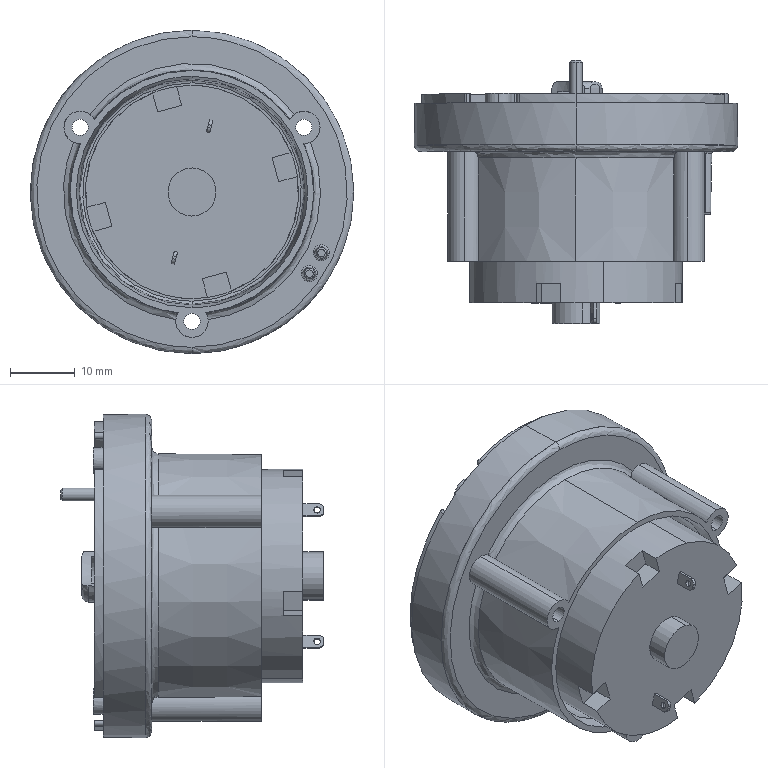Part | SolidWorks | 3 solids | 328 faces | box 50.06 x 40.7 x 50.06 mm | volume 29200 mm3 | cylinder 144 | plane 97 | cone 60 | spline 25 | torus 2 | commonest cylinder face diameters 2 x22 2.5 x18 4 x16 5 x12 1.95 x10 1.087 x8